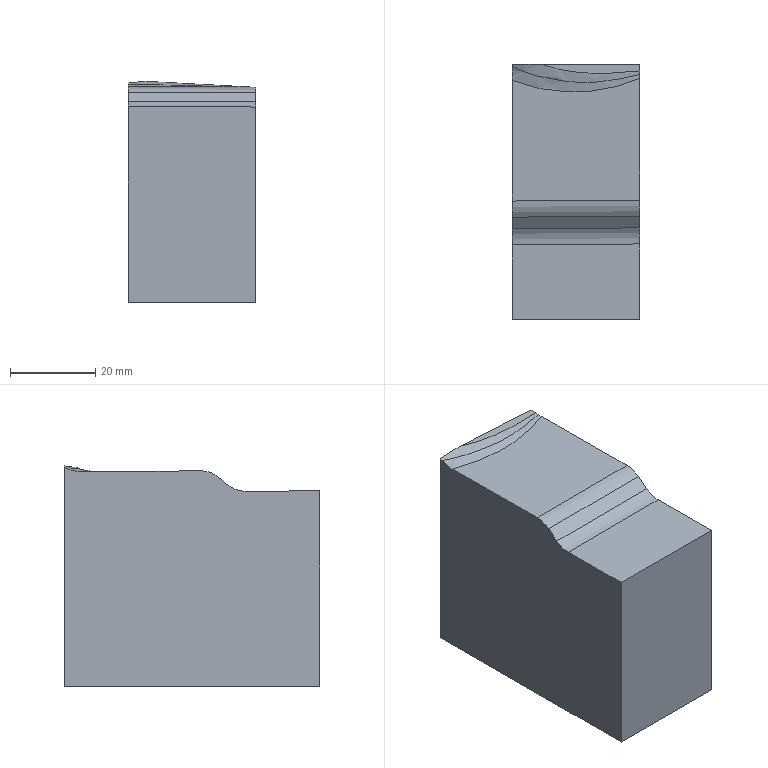Part | NX | features solid 2 | 1 solid | 13 faces | box 30 x 60 x 51.798 mm | volume 87726 mm3 | spline 8 | plane 5
STEP:
#1=CARTESIAN_POINT('',(-180.017,-239.139,60.883));
#2=VERTEX_POINT('',#1);
#3=CARTESIAN_POINT('',(-150.017,-239.139,60.839));
#4=VERTEX_POINT('',#3);
#5=CARTESIAN_POINT('',(-149.942,-239.139,60.838));
#6=DIRECTION('',(1.,0.,-0.001477));
#7=VECTOR('',#6,1000.);
#8=LINE('',#5,#7);
#9=EDGE_CURVE('',#2,#4,#8,.T.);
#10=ORIENTED_EDGE('',*,*,#9,.F.);
#11=CARTESIAN_POINT('',(-180.017,-239.139,15.));
#12=VERTEX_POINT('',#11);
#13=CARTESIAN_POINT('',(-180.017,-239.139,10.));
#14=DIRECTION('',(0.,0.,-1.));
#15=VECTOR('',#14,1000.);
#16=LINE('',#13,#15);
#17=EDGE_CURVE('',#12,#2,#16,.F.);
#18=ORIENTED_EDGE('',*,*,#17,.F.);
#19=CARTESIAN_POINT('',(-150.017,-239.139,15.));
#20=VERTEX_POINT('',#19);
#21=CARTESIAN_POINT('',(-150.017,-239.139,15.));
#22=DIRECTION('',(1.,0.,0.));
#23=VECTOR('',#22,1000.);
#24=LINE('',#21,#23);
#25=EDGE_CURVE('',#20,#12,#24,.F.);
#26=ORIENTED_EDGE('',*,*,#25,.F.);
#27=CARTESIAN_POINT('',(-150.017,-239.139,10.));
#28=DIRECTION('',(0.,0.,-1.));
#29=VECTOR('',#28,1000.);
#30=LINE('',#27,#29);
#31=EDGE_CURVE('',#20,#4,#30,.F.);
#32=ORIENTED_EDGE('',*,*,#31,.T.);
#33=EDGE_LOOP('',(#10,#18,#26,#32));
#34=FACE_BOUND('',#33,.T.);
#35=CARTESIAN_POINT('',(-150.017,-239.139,10.));
#36=DIRECTION('',(0.,-1.,0.));
#37=DIRECTION('',(-1.,0.,0.));
#38=AXIS2_PLACEMENT_3D('',#35,#36,#37);
#39=PLANE('',#38);
#40=ADVANCED_FACE('',(#34),#39,.T.);
#41=CARTESIAN_POINT('',(-180.017,-221.581,60.778));
#42=VERTEX_POINT('',#41);
#43=CARTESIAN_POINT('',(-180.017,-238.836,60.881));
#44=DIRECTION('',(0.,-1.,0.005958));
#45=VECTOR('',#44,1000.);
#46=LINE('',#43,#45);
#47=EDGE_CURVE('',#42,#2,#46,.T.);
#48=ORIENTED_EDGE('',*,*,#47,.F.);
#49=CARTESIAN_POINT('',(-180.017,-217.809,62.084));
#50=VERTEX_POINT('',#49);
#51=CARTESIAN_POINT('',(-180.017,-217.809,62.084));
#52=CARTESIAN_POINT('',(-180.017,-218.876,61.234));
#53=CARTESIAN_POINT('',(-180.017,-220.217,60.77));
#54=CARTESIAN_POINT('',(-180.017,-221.581,60.778));
#55=B_SPLINE_CURVE_WITH_KNOTS('',3,(#51,#52,#53,#54),.UNSPECIFIED.,.F.,.F.,(4,4),(0.00002386,0.004103),.UNSPECIFIED.);
#56=EDGE_CURVE('',#50,#42,#55,.T.);
#57=ORIENTED_EDGE('',*,*,#56,.F.);
#58=CARTESIAN_POINT('',(-180.017,-215.074,64.261));
#59=VERTEX_POINT('',#58);
#60=CARTESIAN_POINT('',(-180.017,-215.074,64.261));
#61=CARTESIAN_POINT('',(-180.017,-215.985,63.535));
#62=CARTESIAN_POINT('',(-180.017,-216.897,62.81));
#63=CARTESIAN_POINT('',(-180.017,-217.809,62.084));
#64=B_SPLINE_CURVE_WITH_KNOTS('',3,(#60,#61,#62,#63),.UNSPECIFIED.,.F.,.F.,(4,4),(0.0001753,0.003671),.UNSPECIFIED.);
#65=EDGE_CURVE('',#59,#50,#64,.T.);
#66=ORIENTED_EDGE('',*,*,#65,.F.);
#67=CARTESIAN_POINT('',(-180.017,-211.301,65.567));
#68=VERTEX_POINT('',#67);
#69=CARTESIAN_POINT('',(-180.017,-215.074,64.261));
#70=CARTESIAN_POINT('',(-180.017,-214.006,65.111));
#71=CARTESIAN_POINT('',(-180.017,-212.665,65.575));
#72=CARTESIAN_POINT('',(-180.017,-211.301,65.567));
#73=B_SPLINE_CURVE_WITH_KNOTS('',3,(#69,#70,#71,#72),.UNSPECIFIED.,.F.,.F.,(4,4),(0.00002386,0.004103),.UNSPECIFIED.);
#74=EDGE_CURVE('',#59,#68,#73,.T.);
#75=ORIENTED_EDGE('',*,*,#74,.T.);
#76=CARTESIAN_POINT('',(-180.017,-182.993,65.398));
#77=VERTEX_POINT('',#76);
#78=CARTESIAN_POINT('',(-180.017,-238.807,65.731));
#79=DIRECTION('',(0.,-1.,0.005958));
#80=VECTOR('',#79,1000.);
#81=LINE('',#78,#80);
#82=EDGE_CURVE('',#77,#68,#81,.T.);
#83=ORIENTED_EDGE('',*,*,#82,.F.);
#84=CARTESIAN_POINT('',(-180.017,-179.72,66.196));
#85=VERTEX_POINT('',#84);
#86=CARTESIAN_POINT('',(-180.017,-182.992,65.398));
#87=CARTESIAN_POINT('',(-180.017,-181.853,65.392));
#88=CARTESIAN_POINT('',(-180.017,-180.719,65.669));
#89=CARTESIAN_POINT('',(-180.017,-179.72,66.196));
#90=B_SPLINE_CURVE_WITH_KNOTS('',3,(#86,#87,#88,#89),.UNSPECIFIED.,.F.,.F.,(4,4),(0.,0.003407),.UNSPECIFIED.);
#91=EDGE_CURVE('',#77,#85,#90,.T.);
#92=ORIENTED_EDGE('',*,*,#91,.T.);
#93=CARTESIAN_POINT('',(-180.017,-179.139,66.47));
#94=VERTEX_POINT('',#93);
#95=CARTESIAN_POINT('',(-180.017,-179.721,66.195));
#96=CARTESIAN_POINT('',(-180.017,-179.531,66.296));
#97=CARTESIAN_POINT('',(-180.017,-179.337,66.387));
#98=CARTESIAN_POINT('',(-180.017,-179.139,66.47));
#99=B_SPLINE_CURVE_WITH_KNOTS('',3,(#95,#96,#97,#98),.UNSPECIFIED.,.F.,.F.,(4,4),(0.,0.0006436),.UNSPECIFIED.);
#100=EDGE_CURVE('',#85,#94,#99,.T.);
#101=ORIENTED_EDGE('',*,*,#100,.T.);
#102=CARTESIAN_POINT('',(-180.017,-179.139,15.));
#103=VERTEX_POINT('',#102);
#104=CARTESIAN_POINT('',(-180.017,-179.139,10.));
#105=DIRECTION('',(0.,0.,-1.));
#106=VECTOR('',#105,1000.);
#107=LINE('',#104,#106);
#108=EDGE_CURVE('',#103,#94,#107,.F.);
#109=ORIENTED_EDGE('',*,*,#108,.F.);
#110=CARTESIAN_POINT('',(-180.017,-239.139,15.));
#111=DIRECTION('',(0.,-1.,0.));
#112=VECTOR('',#111,1000.);
#113=LINE('',#110,#112);
#114=EDGE_CURVE('',#12,#103,#113,.F.);
#115=ORIENTED_EDGE('',*,*,#114,.F.);
#116=ORIENTED_EDGE('',*,*,#17,.T.);
#117=EDGE_LOOP('',(#48,#57,#66,#75,#83,#92,#101,#109,#115,#116));
#118=FACE_BOUND('',#117,.T.);
#119=CARTESIAN_POINT('',(-180.017,-239.139,10.));
#120=DIRECTION('',(-1.,0.,0.));
#121=DIRECTION('',(0.,1.,0.));
#122=AXIS2_PLACEMENT_3D('',#119,#120,#121);
#123=PLANE('',#122);
#124=ADVANCED_FACE('',(#118),#123,.T.);
#125=CARTESIAN_POINT('',(-150.017,-179.139,65.448));
#126=VERTEX_POINT('',#125);
#127=CARTESIAN_POINT('',(-173.414,-179.139,66.725));
#128=VERTEX_POINT('',#127);
#129=CARTESIAN_POINT('',(-146.998,-179.139,65.283));
#130=DIRECTION('',(0.9985,0.,-0.05454));
#131=VECTOR('',#130,1000.);
#132=LINE('',#129,#131);
#133=EDGE_CURVE('',#126,#128,#132,.F.);
#134=ORIENTED_EDGE('',*,*,#133,.F.);
#135=CARTESIAN_POINT('',(-150.017,-179.139,15.));
#136=VERTEX_POINT('',#135);
#137=CARTESIAN_POINT('',(-150.017,-179.139,10.));
#138=DIRECTION('',(0.,0.,-1.));
#139=VECTOR('',#138,1000.);
#140=LINE('',#137,#139);
#141=EDGE_CURVE('',#136,#126,#140,.F.);
#142=ORIENTED_EDGE('',*,*,#141,.F.);
#143=CARTESIAN_POINT('',(-150.017,-179.139,15.));
#144=DIRECTION('',(-1.,0.,0.));
#145=VECTOR('',#144,1000.);
#146=LINE('',#143,#145);
#147=EDGE_CURVE('',#136,#103,#146,.T.);
#148=ORIENTED_EDGE('',*,*,#147,.T.);
#149=ORIENTED_EDGE('',*,*,#108,.T.);
#150=CARTESIAN_POINT('',(-180.017,-179.139,66.47));
#151=CARTESIAN_POINT('',(-177.841,-179.139,66.849));
#152=CARTESIAN_POINT('',(-175.618,-179.139,66.846));
#153=CARTESIAN_POINT('',(-173.413,-179.139,66.725));
#154=B_SPLINE_CURVE_WITH_KNOTS('',3,(#150,#151,#152,#153),.UNSPECIFIED.,.F.,.F.,(4,4),(0.,0.00662),.UNSPECIFIED.);
#155=EDGE_CURVE('',#94,#128,#154,.T.);
#156=ORIENTED_EDGE('',*,*,#155,.T.);
#157=EDGE_LOOP('',(#134,#142,#148,#149,#156));
#158=FACE_BOUND('',#157,.T.);
#159=CARTESIAN_POINT('',(-150.017,-179.139,10.));
#160=DIRECTION('',(0.,-1.,0.));
#161=DIRECTION('',(-1.,0.,0.));
#162=AXIS2_PLACEMENT_3D('',#159,#160,#161);
#163=PLANE('',#162);
#164=ADVANCED_FACE('',(#158),#163,.F.);
#165=CARTESIAN_POINT('',(-150.017,-221.37,60.733));
#166=VERTEX_POINT('',#165);
#167=CARTESIAN_POINT('',(-150.017,-238.836,60.837));
#168=DIRECTION('',(0.,-1.,0.005958));
#169=VECTOR('',#168,1000.);
#170=LINE('',#167,#169);
#171=EDGE_CURVE('',#4,#166,#170,.F.);
#172=ORIENTED_EDGE('',*,*,#171,.F.);
#173=ORIENTED_EDGE('',*,*,#31,.F.);
#174=CARTESIAN_POINT('',(-150.017,-239.139,15.));
#175=DIRECTION('',(0.,1.,0.));
#176=VECTOR('',#175,1000.);
#177=LINE('',#174,#176);
#178=EDGE_CURVE('',#20,#136,#177,.T.);
#179=ORIENTED_EDGE('',*,*,#178,.T.);
#180=ORIENTED_EDGE('',*,*,#141,.T.);
#181=CARTESIAN_POINT('',(-150.017,-180.766,65.461));
#182=VERTEX_POINT('',#181);
#183=CARTESIAN_POINT('',(-150.017,-238.663,65.953));
#184=DIRECTION('',(0.,-1.,0.008496));
#185=VECTOR('',#184,1000.);
#186=LINE('',#183,#185);
#187=EDGE_CURVE('',#182,#126,#186,.F.);
#188=ORIENTED_EDGE('',*,*,#187,.F.);
#189=CARTESIAN_POINT('',(-150.017,-181.592,65.411));
#190=VERTEX_POINT('',#189);
#191=CARTESIAN_POINT('',(-150.017,-180.765,65.461));
#192=CARTESIAN_POINT('',(-150.017,-181.041,65.464));
#193=CARTESIAN_POINT('',(-150.017,-181.318,65.447));
#194=CARTESIAN_POINT('',(-150.017,-181.592,65.411));
#195=B_SPLINE_CURVE_WITH_KNOTS('',3,(#191,#192,#193,#194),.UNSPECIFIED.,.F.,.F.,(4,4),(0.,0.0008294),.UNSPECIFIED.);
#196=EDGE_CURVE('',#182,#190,#195,.T.);
#197=ORIENTED_EDGE('',*,*,#196,.T.);
#198=CARTESIAN_POINT('',(-150.017,-182.555,65.351));
#199=VERTEX_POINT('',#198);
#200=CARTESIAN_POINT('',(-150.017,-181.591,65.411));
#201=CARTESIAN_POINT('',(-150.017,-181.911,65.37));
#202=CARTESIAN_POINT('',(-150.017,-182.232,65.35));
#203=CARTESIAN_POINT('',(-150.017,-182.555,65.351));
#204=B_SPLINE_CURVE_WITH_KNOTS('',3,(#200,#201,#202,#203),.UNSPECIFIED.,.F.,.F.,(4,4),(0.002073,0.003031),.UNSPECIFIED.);
#205=EDGE_CURVE('',#190,#199,#204,.T.);
#206=ORIENTED_EDGE('',*,*,#205,.T.);
#207=CARTESIAN_POINT('',(-150.017,-211.089,65.521));
#208=VERTEX_POINT('',#207);
#209=CARTESIAN_POINT('',(-150.017,-238.807,65.687));
#210=DIRECTION('',(0.,-1.,0.005958));
#211=VECTOR('',#210,1000.);
#212=LINE('',#209,#211);
#213=EDGE_CURVE('',#208,#199,#212,.F.);
#214=ORIENTED_EDGE('',*,*,#213,.F.);
#215=CARTESIAN_POINT('',(-150.017,-214.862,64.216));
#216=VERTEX_POINT('',#215);
#217=CARTESIAN_POINT('',(-150.017,-211.089,65.521));
#218=CARTESIAN_POINT('',(-150.017,-212.454,65.53));
#219=CARTESIAN_POINT('',(-150.017,-213.795,65.066));
#220=CARTESIAN_POINT('',(-150.017,-214.862,64.216));
#221=B_SPLINE_CURVE_WITH_KNOTS('',3,(#217,#218,#219,#220),.UNSPECIFIED.,.F.,.F.,(4,4),(0.00002387,0.004103),.UNSPECIFIED.);
#222=EDGE_CURVE('',#208,#216,#221,.T.);
#223=ORIENTED_EDGE('',*,*,#222,.T.);
#224=CARTESIAN_POINT('',(-150.017,-217.597,62.039));
#225=VERTEX_POINT('',#224);
#226=CARTESIAN_POINT('',(-150.017,-217.597,62.039));
#227=CARTESIAN_POINT('',(-150.017,-216.685,62.764));
#228=CARTESIAN_POINT('',(-150.017,-215.774,63.49));
#229=CARTESIAN_POINT('',(-150.017,-214.862,64.216));
#230=B_SPLINE_CURVE_WITH_KNOTS('',3,(#226,#227,#228,#229),.UNSPECIFIED.,.F.,.F.,(4,4),(0.0005795,0.004075),.UNSPECIFIED.);
#231=EDGE_CURVE('',#225,#216,#230,.T.);
#232=ORIENTED_EDGE('',*,*,#231,.F.);
#233=CARTESIAN_POINT('',(-150.017,-221.37,60.733));
#234=CARTESIAN_POINT('',(-150.017,-220.005,60.725));
#235=CARTESIAN_POINT('',(-150.017,-218.664,61.189));
#236=CARTESIAN_POINT('',(-150.017,-217.597,62.039));
#237=B_SPLINE_CURVE_WITH_KNOTS('',3,(#233,#234,#235,#236),.UNSPECIFIED.,.F.,.F.,(4,4),(0.00002386,0.004103),.UNSPECIFIED.);
#238=EDGE_CURVE('',#166,#225,#237,.T.);
#239=ORIENTED_EDGE('',*,*,#238,.F.);
#240=EDGE_LOOP('',(#172,#173,#179,#180,#188,#197,#206,#214,#223,#232,#239));
#241=FACE_BOUND('',#240,.T.);
#242=CARTESIAN_POINT('',(-150.017,-239.139,10.));
#243=DIRECTION('',(-1.,0.,0.));
#244=DIRECTION('',(0.,1.,0.));
#245=AXIS2_PLACEMENT_3D('',#242,#243,#244);
#246=PLANE('',#245);
#247=ADVANCED_FACE('',(#241),#246,.F.);
#248=ORIENTED_EDGE('',*,*,#147,.F.);
#249=ORIENTED_EDGE('',*,*,#178,.F.);
#250=ORIENTED_EDGE('',*,*,#25,.T.);
#251=ORIENTED_EDGE('',*,*,#114,.T.);
#252=EDGE_LOOP('',(#248,#249,#250,#251));
#253=FACE_BOUND('',#252,.T.);
#254=CARTESIAN_POINT('',(-150.017,-239.139,15.));
#255=DIRECTION('',(0.,0.,-1.));
#256=DIRECTION('',(-1.,0.,0.));
#257=AXIS2_PLACEMENT_3D('',#254,#255,#256);
#258=PLANE('',#257);
#259=ADVANCED_FACE('',(#253),#258,.T.);
#260=ORIENTED_EDGE('',*,*,#47,.T.);
#261=ORIENTED_EDGE('',*,*,#9,.T.);
#262=ORIENTED_EDGE('',*,*,#171,.T.);
#263=CARTESIAN_POINT('',(-180.017,-221.581,60.778));
#264=CARTESIAN_POINT('',(-170.017,-221.511,60.763));
#265=CARTESIAN_POINT('',(-160.017,-221.44,60.748));
#266=CARTESIAN_POINT('',(-150.017,-221.37,60.733));
#267=B_SPLINE_CURVE_WITH_KNOTS('',3,(#263,#264,#265,#266),.UNSPECIFIED.,.F.,.F.,(4,4),(0.7314,0.9716),.UNSPECIFIED.);
#268=EDGE_CURVE('',#42,#166,#267,.T.);
#269=ORIENTED_EDGE('',*,*,#268,.F.);
#270=EDGE_LOOP('',(#260,#261,#262,#269));
#271=FACE_BOUND('',#270,.T.);
#272=CARTESIAN_POINT('',(-180.017,-239.245,60.883));
#273=CARTESIAN_POINT('',(-150.017,-239.246,60.839));
#274=CARTESIAN_POINT('',(-180.017,-221.263,60.776));
#275=CARTESIAN_POINT('',(-150.017,-221.263,60.732));
#276=B_SPLINE_SURFACE_WITH_KNOTS('',1,1,((#272,#273),(#274,#275)),.PLANE_SURF.,.F.,.F.,.F.,(2,2),(2,2),(0.7124,0.7863),(0.7906,0.8614),.PIECEWISE_BEZIER_KNOTS.);
#277=ADVANCED_FACE('',(#271),#276,.F.);
#278=ORIENTED_EDGE('',*,*,#56,.T.);
#279=ORIENTED_EDGE('',*,*,#268,.T.);
#280=ORIENTED_EDGE('',*,*,#238,.T.);
#281=CARTESIAN_POINT('',(-150.017,-217.597,62.039));
#282=CARTESIAN_POINT('',(-160.017,-217.667,62.054));
#283=CARTESIAN_POINT('',(-170.017,-217.738,62.069));
#284=CARTESIAN_POINT('',(-180.017,-217.809,62.084));
#285=B_SPLINE_CURVE_WITH_KNOTS('',3,(#281,#282,#283,#284),.UNSPECIFIED.,.F.,.F.,(4,4),(0.02587,0.2668),.UNSPECIFIED.);
#286=EDGE_CURVE('',#225,#50,#285,.T.);
#287=ORIENTED_EDGE('',*,*,#286,.T.);
#288=EDGE_LOOP('',(#278,#279,#280,#287));
#289=FACE_BOUND('',#288,.T.);
#290=CARTESIAN_POINT('',(-145.715,-221.364,60.726));
#291=CARTESIAN_POINT('',(-272.111,-222.256,60.918));
#292=CARTESIAN_POINT('',(-145.725,-219.963,60.712));
#293=CARTESIAN_POINT('',(-272.121,-220.856,60.904));
#294=CARTESIAN_POINT('',(-145.734,-218.64,61.17));
#295=CARTESIAN_POINT('',(-272.129,-219.532,61.362));
#296=CARTESIAN_POINT('',(-145.74,-217.548,62.047));
#297=CARTESIAN_POINT('',(-272.136,-218.44,62.239));
#298=(BOUNDED_SURFACE()B_SPLINE_SURFACE(3,1,((#290,#291),(#292,#293),(#294,#295),(#296,#297)),.CYLINDRICAL_SURF.,.F.,.F.,.F.)B_SPLINE_SURFACE_WITH_KNOTS((4,4),(2,2),(0.,1.),(0.,1.),.PIECEWISE_BEZIER_KNOTS.)GEOMETRIC_REPRESENTATION_ITEM()RATIONAL_B_SPLINE_SURFACE(((1.,1.),(0.9611,0.9611),(0.9611,0.9611),(1.,1.)))REPRESENTATION_ITEM('')SURFACE());
#299=ADVANCED_FACE('',(#289),#298,.T.);
#300=ORIENTED_EDGE('',*,*,#133,.T.);
#301=CARTESIAN_POINT('',(-150.017,-180.768,65.461));
#302=CARTESIAN_POINT('',(-150.256,-180.779,65.475));
#303=CARTESIAN_POINT('',(-150.803,-180.812,65.505));
#304=CARTESIAN_POINT('',(-151.722,-180.89,65.556));
#305=CARTESIAN_POINT('',(-153.071,-181.019,65.63));
#306=CARTESIAN_POINT('',(-153.921,-181.097,65.677));
#307=CARTESIAN_POINT('',(-154.388,-181.14,65.703));
#308=CARTESIAN_POINT('',(-154.535,-181.154,65.711));
#309=CARTESIAN_POINT('',(-154.612,-181.16,65.716));
#310=CARTESIAN_POINT('',(-154.926,-181.186,65.733));
#311=CARTESIAN_POINT('',(-155.233,-181.21,65.75));
#312=CARTESIAN_POINT('',(-155.765,-181.249,65.779));
#313=CARTESIAN_POINT('',(-156.658,-181.306,65.829));
#314=CARTESIAN_POINT('',(-157.897,-181.365,65.897));
#315=CARTESIAN_POINT('',(-159.071,-181.39,65.961));
#316=CARTESIAN_POINT('',(-159.966,-181.39,66.01));
#317=CARTESIAN_POINT('',(-160.987,-181.375,66.066));
#318=CARTESIAN_POINT('',(-162.695,-181.308,66.158));
#319=CARTESIAN_POINT('',(-165.119,-181.094,66.289));
#320=CARTESIAN_POINT('',(-167.936,-180.65,66.439));
#321=CARTESIAN_POINT('',(-170.684,-180.017,66.584));
#322=CARTESIAN_POINT('',(-172.52,-179.452,66.679));
#323=CARTESIAN_POINT('',(-173.414,-179.139,66.725));
#324=B_SPLINE_CURVE_WITH_KNOTS('',3,(#301,#302,#303,#304,#305,#306,#307,#308,#309,#310,#311,#312,#313,#314,#315,#316,#317,#318,#319,#320,#321,#322,#323),.UNSPECIFIED.,.F.,.F.,(4,1,1,1,1,1,1,1,1,1,1,1,1,1,1,1,1,1,1,1,4),(0.0255,0.04302,0.06055,0.07808,0.0956,0.1131,0.1219,0.1263,0.1307,0.1394,0.1482,0.1657,0.2008,0.2358,0.2533,0.2709,0.3059,0.376,0.4461,0.5163,0.5864),.UNSPECIFIED.);
#325=EDGE_CURVE('',#182,#128,#324,.T.);
#326=ORIENTED_EDGE('',*,*,#325,.F.);
#327=ORIENTED_EDGE('',*,*,#187,.T.);
#328=EDGE_LOOP('',(#300,#326,#327));
#329=FACE_BOUND('',#328,.T.);
#330=CARTESIAN_POINT('',(-149.872,-181.391,65.459));
#331=CARTESIAN_POINT('',(-149.877,-179.08,65.439));
#332=CARTESIAN_POINT('',(-173.549,-181.436,66.752));
#333=CARTESIAN_POINT('',(-173.555,-179.125,66.733));
#334=B_SPLINE_SURFACE_WITH_KNOTS('',1,1,((#330,#331),(#332,#333)),.PLANE_SURF.,.F.,.F.,.F.,(2,2),(2,2),(0.6787,0.8383),(0.3159,0.3381),.PIECEWISE_BEZIER_KNOTS.);
#335=ADVANCED_FACE('',(#329),#334,.F.);
#336=ORIENTED_EDGE('',*,*,#65,.T.);
#337=ORIENTED_EDGE('',*,*,#286,.F.);
#338=ORIENTED_EDGE('',*,*,#231,.T.);
#339=CARTESIAN_POINT('',(-180.017,-215.074,64.261));
#340=CARTESIAN_POINT('',(-170.017,-215.003,64.246));
#341=CARTESIAN_POINT('',(-160.017,-214.933,64.231));
#342=CARTESIAN_POINT('',(-150.017,-214.862,64.216));
#343=B_SPLINE_CURVE_WITH_KNOTS('',3,(#339,#340,#341,#342),.UNSPECIFIED.,.F.,.F.,(4,4),(0.7351,0.9761),.UNSPECIFIED.);
#344=EDGE_CURVE('',#59,#216,#343,.T.);
#345=ORIENTED_EDGE('',*,*,#344,.F.);
#346=EDGE_LOOP('',(#336,#337,#338,#345));
#347=FACE_BOUND('',#346,.T.);
#348=CARTESIAN_POINT('',(-180.017,-217.826,62.07));
#349=CARTESIAN_POINT('',(-150.017,-217.721,61.939));
#350=CARTESIAN_POINT('',(-180.017,-214.949,64.36));
#351=CARTESIAN_POINT('',(-150.017,-214.845,64.229));
#352=B_SPLINE_SURFACE_WITH_KNOTS('',1,1,((#348,#349),(#350,#351)),.PLANE_SURF.,.F.,.F.,.F.,(2,2),(2,2),(0.1022,0.9961),(0.7315,0.9686),.PIECEWISE_BEZIER_KNOTS.);
#353=ADVANCED_FACE('',(#347),#352,.F.);
#354=CARTESIAN_POINT('',(-180.018,-179.721,66.195));
#355=CARTESIAN_POINT('',(-175.375,-181.917,66.093));
#356=CARTESIAN_POINT('',(-167.763,-183.759,65.911));
#357=CARTESIAN_POINT('',(-157.489,-183.33,65.634));
#358=CARTESIAN_POINT('',(-152.488,-182.163,65.488));
#359=CARTESIAN_POINT('',(-150.017,-181.592,65.411));
#360=B_SPLINE_CURVE_WITH_KNOTS('',3,(#354,#355,#356,#357,#358,#359),.UNSPECIFIED.,.F.,.F.,(4,1,1,4),(0.2757,0.6279,0.804,0.9801),.UNSPECIFIED.);
#361=EDGE_CURVE('',#85,#190,#360,.T.);
#362=ORIENTED_EDGE('',*,*,#361,.T.);
#363=ORIENTED_EDGE('',*,*,#196,.F.);
#364=ORIENTED_EDGE('',*,*,#325,.T.);
#365=ORIENTED_EDGE('',*,*,#155,.F.);
#366=ORIENTED_EDGE('',*,*,#100,.F.);
#367=EDGE_LOOP('',(#362,#363,#364,#365,#366));
#368=FACE_BOUND('',#367,.T.);
#369=CARTESIAN_POINT('',(-149.827,-180.757,65.451));
#370=CARTESIAN_POINT('',(-149.822,-180.915,65.452));
#371=CARTESIAN_POINT('',(-149.817,-181.072,65.448));
#372=CARTESIAN_POINT('',(-149.812,-181.23,65.439));
#373=CARTESIAN_POINT('',(-149.808,-181.387,65.424));
#374=CARTESIAN_POINT('',(-149.804,-181.543,65.405));
#375=CARTESIAN_POINT('',(-150.247,-180.771,65.474));
#376=CARTESIAN_POINT('',(-150.237,-180.944,65.475));
#377=CARTESIAN_POINT('',(-150.227,-181.117,65.47));
#378=CARTESIAN_POINT('',(-150.218,-181.289,65.458));
#379=CARTESIAN_POINT('',(-150.209,-181.461,65.441));
#380=CARTESIAN_POINT('',(-150.2,-181.632,65.417));
#381=CARTESIAN_POINT('',(-150.661,-180.8,65.497));
#382=CARTESIAN_POINT('',(-150.647,-180.986,65.498));
#383=CARTESIAN_POINT('',(-150.634,-181.172,65.491));
#384=CARTESIAN_POINT('',(-150.621,-181.358,65.478));
#385=CARTESIAN_POINT('',(-150.608,-181.544,65.457));
#386=CARTESIAN_POINT('',(-150.596,-181.728,65.429));
#387=CARTESIAN_POINT('',(-151.072,-180.832,65.52));
#388=CARTESIAN_POINT('',(-151.055,-181.031,65.52));
#389=CARTESIAN_POINT('',(-151.039,-181.23,65.513));
#390=CARTESIAN_POINT('',(-151.023,-181.429,65.497));
#391=CARTESIAN_POINT('',(-151.008,-181.626,65.473));
#392=CARTESIAN_POINT('',(-150.993,-181.823,65.441));
#393=CARTESIAN_POINT('',(-152.287,-180.942,65.587));
#394=CARTESIAN_POINT('',(-152.263,-181.176,65.588));
#395=CARTESIAN_POINT('',(-152.24,-181.41,65.577));
#396=CARTESIAN_POINT('',(-152.218,-181.644,65.555));
#397=CARTESIAN_POINT('',(-152.197,-181.876,65.522));
#398=CARTESIAN_POINT('',(-152.176,-182.107,65.477));
#399=CARTESIAN_POINT('',(-153.483,-181.062,65.653));
#400=CARTESIAN_POINT('',(-153.458,-181.326,65.654));
#401=CARTESIAN_POINT('',(-153.433,-181.591,65.64));
#402=CARTESIAN_POINT('',(-153.409,-181.855,65.612));
#403=CARTESIAN_POINT('',(-153.386,-182.116,65.569));
#404=CARTESIAN_POINT('',(-153.364,-182.375,65.512));
#405=CARTESIAN_POINT('',(-154.274,-181.136,65.697));
#406=CARTESIAN_POINT('',(-154.249,-181.419,65.698));
#407=CARTESIAN_POINT('',(-154.224,-181.703,65.682));
#408=CARTESIAN_POINT('',(-154.2,-181.985,65.65));
#409=CARTESIAN_POINT('',(-154.178,-182.265,65.601));
#410=CARTESIAN_POINT('',(-154.157,-182.541,65.536));
#411=CARTESIAN_POINT('',(-155.997,-181.278,65.792));
#412=CARTESIAN_POINT('',(-155.975,-181.6,65.794));
#413=CARTESIAN_POINT('',(-155.954,-181.922,65.774));
#414=CARTESIAN_POINT('',(-155.934,-182.243,65.732));
#415=CARTESIAN_POINT('',(-155.915,-182.56,65.67));
#416=CARTESIAN_POINT('',(-155.898,-182.871,65.586));
#417=CARTESIAN_POINT('',(-157.709,-181.365,65.887));
#418=CARTESIAN_POINT('',(-157.694,-181.721,65.889));
#419=CARTESIAN_POINT('',(-157.682,-182.078,65.865));
#420=CARTESIAN_POINT('',(-157.671,-182.433,65.814));
#421=CARTESIAN_POINT('',(-157.661,-182.782,65.738));
#422=CARTESIAN_POINT('',(-157.653,-183.124,65.636));
#423=CARTESIAN_POINT('',(-158.635,-181.392,65.937));
#424=CARTESIAN_POINT('',(-158.627,-181.766,65.94));
#425=CARTESIAN_POINT('',(-158.62,-182.141,65.914));
#426=CARTESIAN_POINT('',(-158.615,-182.513,65.858));
#427=CARTESIAN_POINT('',(-158.612,-182.879,65.774));
#428=CARTESIAN_POINT('',(-158.61,-183.236,65.663));
#429=CARTESIAN_POINT('',(-161.345,-181.41,66.086));
#430=CARTESIAN_POINT('',(-161.357,-181.834,66.09));
#431=CARTESIAN_POINT('',(-161.371,-182.258,66.057));
#432=CARTESIAN_POINT('',(-161.388,-182.678,65.987));
#433=CARTESIAN_POINT('',(-161.406,-183.09,65.881));
#434=CARTESIAN_POINT('',(-161.426,-183.489,65.74));
#435=CARTESIAN_POINT('',(-164.025,-181.237,66.23));
#436=CARTESIAN_POINT('',(-164.067,-181.703,66.237));
#437=CARTESIAN_POINT('',(-164.112,-182.168,66.198));
#438=CARTESIAN_POINT('',(-164.159,-182.629,66.114));
#439=CARTESIAN_POINT('',(-164.207,-183.078,65.986));
#440=CARTESIAN_POINT('',(-164.257,-183.511,65.816));
#441=CARTESIAN_POINT('',(-165.776,-181.032,66.324));
#442=CARTESIAN_POINT('',(-165.842,-181.522,66.332));
#443=CARTESIAN_POINT('',(-165.91,-182.013,66.289));
#444=CARTESIAN_POINT('',(-165.98,-182.497,66.196));
#445=CARTESIAN_POINT('',(-166.052,-182.968,66.053));
#446=CARTESIAN_POINT('',(-166.123,-183.419,65.864));
#447=CARTESIAN_POINT('',(-169.578,-180.381,66.527));
#448=CARTESIAN_POINT('',(-169.701,-180.918,66.538));
#449=CARTESIAN_POINT('',(-169.828,-181.455,66.487));
#450=CARTESIAN_POINT('',(-169.955,-181.984,66.373));
#451=CARTESIAN_POINT('',(-170.082,-182.495,66.199));
#452=CARTESIAN_POINT('',(-170.207,-182.979,65.968));
#453=CARTESIAN_POINT('',(-173.246,-179.286,66.718));
#454=CARTESIAN_POINT('',(-173.437,-179.854,66.733));
#455=CARTESIAN_POINT('',(-173.633,-180.422,66.674));
#456=CARTESIAN_POINT('',(-173.829,-180.979,66.54));
#457=CARTESIAN_POINT('',(-174.022,-181.514,66.335));
#458=CARTESIAN_POINT('',(-174.206,-182.015,66.064));
#459=CARTESIAN_POINT('',(-175.193,-178.557,66.818));
#460=CARTESIAN_POINT('',(-175.425,-179.137,66.835));
#461=CARTESIAN_POINT('',(-175.662,-179.717,66.772));
#462=CARTESIAN_POINT('',(-175.898,-180.285,66.628));
#463=CARTESIAN_POINT('',(-176.127,-180.828,66.407));
#464=CARTESIAN_POINT('',(-176.346,-181.334,66.114));
#465=CARTESIAN_POINT('',(-177.079,-177.7,66.913));
#466=CARTESIAN_POINT('',(-177.353,-178.286,66.933));
#467=CARTESIAN_POINT('',(-177.632,-178.873,66.866));
#468=CARTESIAN_POINT('',(-177.909,-179.447,66.712));
#469=CARTESIAN_POINT('',(-178.177,-179.993,66.475));
#470=CARTESIAN_POINT('',(-178.431,-180.499,66.161));
#471=CARTESIAN_POINT('',(-178.89,-176.719,67.004));
#472=CARTESIAN_POINT('',(-179.207,-177.307,67.026));
#473=CARTESIAN_POINT('',(-179.529,-177.895,66.956));
#474=CARTESIAN_POINT('',(-179.848,-178.469,66.792));
#475=CARTESIAN_POINT('',(-180.156,-179.014,66.539));
#476=CARTESIAN_POINT('',(-180.444,-179.516,66.205));
#477=B_SPLINE_SURFACE_WITH_KNOTS('',5,5,((#369,#370,#371,#372,#373,#374),(#375,#376,#377,#378,#379,#380),(#381,#382,#383,#384,#385,#386),(#387,#388,#389,#390,#391,#392),(#393,#394,#395,#396,#397,#398),(#399,#400,#401,#402,#403,#404),(#405,#406,#407,#408,#409,#410),(#411,#412,#413,#414,#415,#416),(#417,#418,#419,#420,#421,#422),(#423,#424,#425,#426,#427,#428),(#429,#430,#431,#432,#433,#434),(#435,#436,#437,#438,#439,#440),(#441,#442,#443,#444,#445,#446),(#447,#448,#449,#450,#451,#452),(#453,#454,#455,#456,#457,#458),(#459,#460,#461,#462,#463,#464),(#465,#466,#467,#468,#469,#470),(#471,#472,#473,#474,#475,#476)),.UNSPECIFIED.,.F.,.F.,.F.,(6,3,3,3,3,6),(6,6),(0.01483,0.06188,0.1549,0.2653,0.4791,0.7352),(0.,1.),.UNSPECIFIED.);
#478=ADVANCED_FACE('',(#368),#477,.T.);
#479=ORIENTED_EDGE('',*,*,#344,.T.);
#480=ORIENTED_EDGE('',*,*,#222,.F.);
#481=CARTESIAN_POINT('',(-180.017,-211.301,65.567));
#482=CARTESIAN_POINT('',(-170.017,-211.23,65.552));
#483=CARTESIAN_POINT('',(-160.017,-211.16,65.537));
#484=CARTESIAN_POINT('',(-150.017,-211.089,65.521));
#485=B_SPLINE_CURVE_WITH_KNOTS('',3,(#481,#482,#483,#484),.UNSPECIFIED.,.F.,.F.,(4,4),(0.7372,0.9787),.UNSPECIFIED.);
#486=EDGE_CURVE('',#68,#208,#485,.T.);
#487=ORIENTED_EDGE('',*,*,#486,.F.);
#488=ORIENTED_EDGE('',*,*,#74,.F.);
#489=EDGE_LOOP('',(#479,#480,#487,#488));
#490=FACE_BOUND('',#489,.T.);
#491=CARTESIAN_POINT('',(-149.837,-211.088,65.521));
#492=CARTESIAN_POINT('',(-180.222,-211.302,65.567));
#493=CARTESIAN_POINT('',(-149.827,-212.471,65.529));
#494=CARTESIAN_POINT('',(-180.212,-212.686,65.576));
#495=CARTESIAN_POINT('',(-149.819,-213.778,65.077));
#496=CARTESIAN_POINT('',(-180.204,-213.993,65.123));
#497=CARTESIAN_POINT('',(-149.813,-214.861,64.215));
#498=CARTESIAN_POINT('',(-180.197,-215.075,64.261));
#499=(BOUNDED_SURFACE()B_SPLINE_SURFACE(3,1,((#491,#492),(#493,#494),(#495,#496),(#497,#498)),.CYLINDRICAL_SURF.,.F.,.F.,.F.)B_SPLINE_SURFACE_WITH_KNOTS((4,4),(2,2),(0.006047,0.994),(0.02767,0.2656),.PIECEWISE_BEZIER_KNOTS.)GEOMETRIC_REPRESENTATION_ITEM()RATIONAL_B_SPLINE_SURFACE(((0.9993,0.9993),(0.9613,0.9613),(0.9613,0.9613),(0.9993,0.9993)))REPRESENTATION_ITEM('')SURFACE());
#500=ADVANCED_FACE('',(#490),#499,.F.);
#501=CARTESIAN_POINT('',(-180.017,-182.992,65.398));
#502=CARTESIAN_POINT('',(-175.181,-184.884,65.403));
#503=CARTESIAN_POINT('',(-164.82,-186.719,65.398));
#504=CARTESIAN_POINT('',(-154.675,-184.535,65.37));
#505=CARTESIAN_POINT('',(-150.017,-182.555,65.351));
#506=B_SPLINE_CURVE_WITH_KNOTS('',3,(#501,#502,#503,#504,#505),.UNSPECIFIED.,.F.,.F.,(4,1,4),(0.3068,0.6398,0.9728),.UNSPECIFIED.);
#507=EDGE_CURVE('',#77,#199,#506,.T.);
#508=ORIENTED_EDGE('',*,*,#507,.T.);
#509=ORIENTED_EDGE('',*,*,#205,.F.);
#510=ORIENTED_EDGE('',*,*,#361,.F.);
#511=ORIENTED_EDGE('',*,*,#91,.F.);
#512=EDGE_LOOP('',(#508,#509,#510,#511));
#513=FACE_BOUND('',#512,.T.);
#514=CARTESIAN_POINT('',(-150.79,-179.375,66.271));
#515=CARTESIAN_POINT('',(-150.558,-179.901,65.909));
#516=CARTESIAN_POINT('',(-150.305,-180.475,65.628));
#517=CARTESIAN_POINT('',(-150.038,-181.081,65.439));
#518=CARTESIAN_POINT('',(-149.763,-181.703,65.346));
#519=CARTESIAN_POINT('',(-149.488,-182.325,65.349));
#520=CARTESIAN_POINT('',(-154.448,-181.019,66.271));
#521=CARTESIAN_POINT('',(-154.275,-181.569,65.915));
#522=CARTESIAN_POINT('',(-154.087,-182.166,65.639));
#523=CARTESIAN_POINT('',(-153.888,-182.797,65.453));
#524=CARTESIAN_POINT('',(-153.684,-183.445,65.362));
#525=CARTESIAN_POINT('',(-153.479,-184.091,65.366));
#526=CARTESIAN_POINT('',(-158.352,-182.171,66.268));
#527=CARTESIAN_POINT('',(-158.241,-182.735,65.918));
#528=CARTESIAN_POINT('',(-158.121,-183.347,65.647));
#529=CARTESIAN_POINT('',(-157.994,-183.993,65.465));
#530=CARTESIAN_POINT('',(-157.863,-184.655,65.376));
#531=CARTESIAN_POINT('',(-157.733,-185.317,65.379));
#532=CARTESIAN_POINT('',(-162.415,-182.778,66.262));
#533=CARTESIAN_POINT('',(-162.368,-183.347,65.918));
#534=CARTESIAN_POINT('',(-162.317,-183.964,65.652));
#535=CARTESIAN_POINT('',(-162.263,-184.615,65.473));
#536=CARTESIAN_POINT('',(-162.207,-185.282,65.386));
#537=CARTESIAN_POINT('',(-162.151,-185.948,65.39));
#538=CARTESIAN_POINT('',(-168.527,-182.826,66.248));
#539=CARTESIAN_POINT('',(-168.573,-183.39,65.913));
#540=CARTESIAN_POINT('',(-168.624,-184.,65.655));
#541=CARTESIAN_POINT('',(-168.677,-184.642,65.48));
#542=CARTESIAN_POINT('',(-168.731,-185.3,65.395));
#543=CARTESIAN_POINT('',(-168.785,-185.958,65.399));
#544=CARTESIAN_POINT('',(-174.519,-181.613,66.228));
#545=CARTESIAN_POINT('',(-174.656,-182.153,65.901));
#546=CARTESIAN_POINT('',(-174.803,-182.736,65.649));
#547=CARTESIAN_POINT('',(-174.957,-183.349,65.48));
#548=CARTESIAN_POINT('',(-175.116,-183.976,65.397));
#549=CARTESIAN_POINT('',(-175.274,-184.603,65.401));
#550=CARTESIAN_POINT('',(-176.447,-181.083,66.221));
#551=CARTESIAN_POINT('',(-176.612,-181.614,65.897));
#552=CARTESIAN_POINT('',(-176.79,-182.186,65.647));
#553=CARTESIAN_POINT('',(-176.977,-182.787,65.479));
#554=CARTESIAN_POINT('',(-177.169,-183.403,65.397));
#555=CARTESIAN_POINT('',(-177.36,-184.017,65.401));
#556=CARTESIAN_POINT('',(-178.338,-180.422,66.213));
#557=CARTESIAN_POINT('',(-178.531,-180.941,65.892));
#558=CARTESIAN_POINT('',(-178.739,-181.501,65.643));
#559=CARTESIAN_POINT('',(-178.957,-182.088,65.477));
#560=CARTESIAN_POINT('',(-179.18,-182.689,65.395));
#561=CARTESIAN_POINT('',(-179.404,-183.29,65.399));
#562=CARTESIAN_POINT('',(-180.178,-179.633,66.205));
#563=CARTESIAN_POINT('',(-180.398,-180.139,65.886));
#564=CARTESIAN_POINT('',(-180.635,-180.683,65.639));
#565=CARTESIAN_POINT('',(-180.884,-181.255,65.474));
#566=CARTESIAN_POINT('',(-181.138,-181.84,65.393));
#567=CARTESIAN_POINT('',(-181.392,-182.424,65.397));
#568=B_SPLINE_SURFACE_WITH_KNOTS('',5,5,((#514,#515,#516,#517,#518,#519),(#520,#521,#522,#523,#524,#525),(#526,#527,#528,#529,#530,#531),(#532,#533,#534,#535,#536,#537),(#538,#539,#540,#541,#542,#543),(#544,#545,#546,#547,#548,#549),(#550,#551,#552,#553,#554,#555),(#556,#557,#558,#559,#560,#561),(#562,#563,#564,#565,#566,#567)),.UNSPECIFIED.,.F.,.F.,.F.,(6,3,6),(6,6),(0.01454,0.4934,0.7249),(0.1316,1.),.UNSPECIFIED.);
#569=ADVANCED_FACE('',(#513),#568,.T.);
#570=ORIENTED_EDGE('',*,*,#82,.T.);
#571=ORIENTED_EDGE('',*,*,#486,.T.);
#572=ORIENTED_EDGE('',*,*,#213,.T.);
#573=ORIENTED_EDGE('',*,*,#507,.F.);
#574=EDGE_LOOP('',(#570,#571,#572,#573));
#575=FACE_BOUND('',#574,.T.);
#576=CARTESIAN_POINT('',(-180.198,-211.473,65.568));
#577=CARTESIAN_POINT('',(-149.837,-211.474,65.524));
#578=CARTESIAN_POINT('',(-180.198,-182.382,65.395));
#579=CARTESIAN_POINT('',(-149.837,-182.382,65.35));
#580=B_SPLINE_SURFACE_WITH_KNOTS('',1,1,((#576,#577),(#578,#579)),.PLANE_SURF.,.F.,.F.,.F.,(2,2),(2,2),(0.01908,0.806),(0.7382,0.9748),.PIECEWISE_BEZIER_KNOTS.);
#581=ADVANCED_FACE('',(#575),#580,.F.);
#582=CLOSED_SHELL('',(#40,#124,#164,#247,#259,#277,#299,#335,#353,#478,#500,#569,#581));
#583=MANIFOLD_SOLID_BREP('',#582);
#584=(LENGTH_UNIT()NAMED_UNIT(*)SI_UNIT(.MILLI.,.METRE.));
#585=UNCERTAINTY_MEASURE_WITH_UNIT(LENGTH_MEASURE(0.05414),#584,'','');
#586=(NAMED_UNIT(*)PLANE_ANGLE_UNIT()SI_UNIT($,.RADIAN.));
#587=(NAMED_UNIT(*)SI_UNIT($,.STERADIAN.)SOLID_ANGLE_UNIT());
#588=(GEOMETRIC_REPRESENTATION_CONTEXT(3)GLOBAL_UNCERTAINTY_ASSIGNED_CONTEXT((#585))GLOBAL_UNIT_ASSIGNED_CONTEXT((#584,#586,#587))REPRESENTATION_CONTEXT('',''));
#589=ADVANCED_BREP_SHAPE_REPRESENTATION('',(#583),#588);